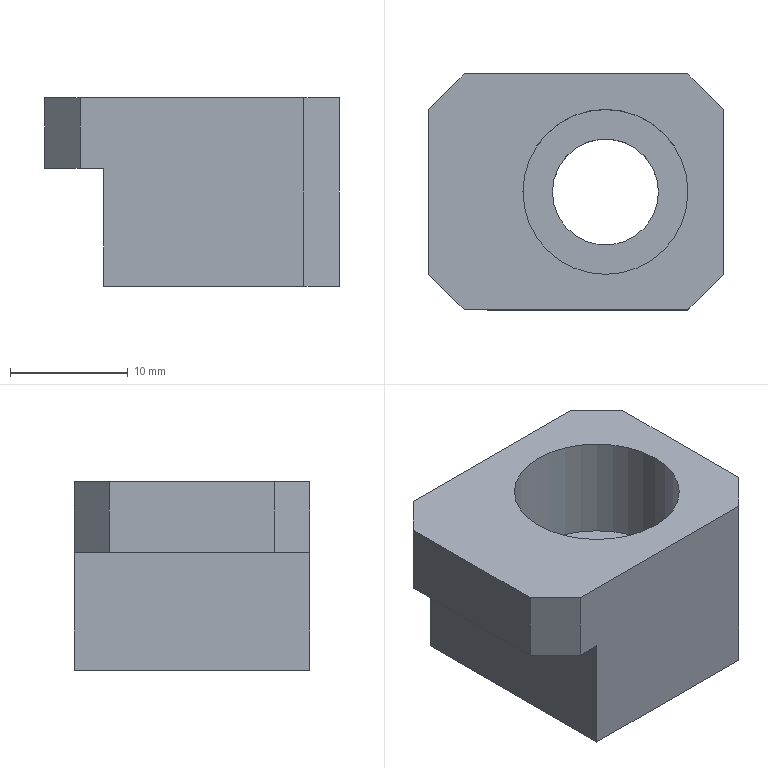Part | STEP file | gslz 2016.10.28-10_id1570_x_t | 1 solid | 15 faces | box 25 x 20 x 16 mm | volume 4971 mm3 | plane 13 | cylinder 2 | commonest cylinder face diameters 9 x1 14 x1
STEP:
#1=CARTESIAN_POINT('',(0.,0.,0.));
#2=DIRECTION('',(0.,0.,1.));
#3=DIRECTION('',(1.,0.,0.));
#4=AXIS2_PLACEMENT_3D('',#1,#2,#3);
#5=CARTESIAN_POINT('',(-846.5,210.,65.));
#6=VERTEX_POINT('',#5);
#7=CARTESIAN_POINT('',(-851.,210.,65.));
#8=DIRECTION('',(0.,0.,1.));
#9=DIRECTION('',(1.,0.,0.));
#10=AXIS2_PLACEMENT_3D('',#7,#8,#9);
#11=CIRCLE('',#10,4.5);
#12=CARTESIAN_POINT('',(-858.5,212.5,65.));
#13=DIRECTION('',(0.,0.,-1.));
#14=DIRECTION('',(1.,0.,0.));
#15=AXIS2_PLACEMENT_3D('',#12,#13,#14);
#16=PLANE('',#15);
#17=CARTESIAN_POINT('',(12.,2.5));
#18=CARTESIAN_POINT('',(12.,-5.294));
#19=CARTESIAN_POINT('',(5.25,-1.397));
#20=CARTESIAN_POINT('',(-1.5,2.5));
#21=CARTESIAN_POINT('',(5.25,6.397));
#22=CARTESIAN_POINT('',(12.,10.294));
#23=CARTESIAN_POINT('',(12.,2.5));
#24=(BOUNDED_CURVE()B_SPLINE_CURVE(2,(#17,#18,#19,#20,#21,#22,#23),.UNSPECIFIED.,.T.,.F.)B_SPLINE_CURVE_WITH_KNOTS((1,2,2,2,2,1),(-2.094,0.,2.094,4.189,6.283,8.378),.UNSPECIFIED.)CURVE()GEOMETRIC_REPRESENTATION_ITEM()RATIONAL_B_SPLINE_CURVE((1.,0.5,1.,0.5,1.,0.5,1.))REPRESENTATION_ITEM(''));
#25=(GEOMETRIC_REPRESENTATION_CONTEXT(2)PARAMETRIC_REPRESENTATION_CONTEXT()REPRESENTATION_CONTEXT('',''));
#26=DEFINITIONAL_REPRESENTATION('',(#24),#25);
#27=PCURVE('',#16,#26);
#28=CARTESIAN_POINT('',(-851.,210.,66.));
#29=DIRECTION('',(0.,0.,-1.));
#30=DIRECTION('',(0.,-1.,0.));
#31=AXIS2_PLACEMENT_3D('',#28,#29,#30);
#32=CYLINDRICAL_SURFACE('',#31,4.5);
#33=CARTESIAN_POINT('',(10.996,1.));
#34=DIRECTION('',(-1.,0.));
#35=VECTOR('',#34,1.);
#36=LINE('',#33,#35);
#37=(GEOMETRIC_REPRESENTATION_CONTEXT(2)PARAMETRIC_REPRESENTATION_CONTEXT()REPRESENTATION_CONTEXT('',''));
#38=DEFINITIONAL_REPRESENTATION('',(#36),#37);
#39=PCURVE('',#32,#38);
#40=SURFACE_CURVE('',#11,(#27,#39),.PCURVE_S1.);
#41=EDGE_CURVE('',#6,#6,#40,.T.);
#42=ORIENTED_EDGE('',*,*,#41,.T.);
#43=EDGE_LOOP('',(#42));
#44=FACE_BOUND('',#43,.T.);
#45=CARTESIAN_POINT('',(-841.,217.,65.));
#46=VERTEX_POINT('',#45);
#47=CARTESIAN_POINT('',(-841.,203.,65.));
#48=VERTEX_POINT('',#47);
#49=CARTESIAN_POINT('',(-841.,212.5,65.));
#50=DIRECTION('',(0.,-1.,0.));
#51=VECTOR('',#50,1.);
#52=LINE('',#49,#51);
#53=CARTESIAN_POINT('',(17.5,0.));
#54=DIRECTION('',(0.,1.));
#55=VECTOR('',#54,1.);
#56=LINE('',#53,#55);
#57=(GEOMETRIC_REPRESENTATION_CONTEXT(2)PARAMETRIC_REPRESENTATION_CONTEXT()REPRESENTATION_CONTEXT('',''));
#58=DEFINITIONAL_REPRESENTATION('',(#56),#57);
#59=PCURVE('',#16,#58);
#60=CARTESIAN_POINT('',(-841.,212.5,76.));
#61=DIRECTION('',(1.,0.,0.));
#62=DIRECTION('',(0.,0.,1.));
#63=AXIS2_PLACEMENT_3D('',#60,#61,#62);
#64=PLANE('',#63);
#65=CARTESIAN_POINT('',(-11.,0.));
#66=DIRECTION('',(0.,1.));
#67=VECTOR('',#66,1.);
#68=LINE('',#65,#67);
#69=(GEOMETRIC_REPRESENTATION_CONTEXT(2)PARAMETRIC_REPRESENTATION_CONTEXT()REPRESENTATION_CONTEXT('',''));
#70=DEFINITIONAL_REPRESENTATION('',(#68),#69);
#71=PCURVE('',#64,#70);
#72=SURFACE_CURVE('',#52,(#59,#71),.PCURVE_S1.);
#73=EDGE_CURVE('',#46,#48,#72,.T.);
#74=ORIENTED_EDGE('',*,*,#73,.T.);
#75=CARTESIAN_POINT('',(-844.,200.,65.));
#76=VERTEX_POINT('',#75);
#77=CARTESIAN_POINT('',(-845.,199.,65.));
#78=DIRECTION('',(0.7071,0.7071,0.));
#79=VECTOR('',#78,1.);
#80=LINE('',#77,#79);
#81=CARTESIAN_POINT('',(13.5,13.5));
#82=DIRECTION('',(0.7071,-0.7071));
#83=VECTOR('',#82,1.);
#84=LINE('',#81,#83);
#85=(GEOMETRIC_REPRESENTATION_CONTEXT(2)PARAMETRIC_REPRESENTATION_CONTEXT()REPRESENTATION_CONTEXT('',''));
#86=DEFINITIONAL_REPRESENTATION('',(#84),#85);
#87=PCURVE('',#16,#86);
#88=CARTESIAN_POINT('',(-841.,203.,76.));
#89=DIRECTION('',(-0.7071,0.7071,0.));
#90=DIRECTION('',(0.,0.,1.));
#91=AXIS2_PLACEMENT_3D('',#88,#89,#90);
#92=PLANE('',#91);
#93=CARTESIAN_POINT('',(-11.,-5.657));
#94=DIRECTION('',(0.,1.));
#95=VECTOR('',#94,1.);
#96=LINE('',#93,#95);
#97=(GEOMETRIC_REPRESENTATION_CONTEXT(2)PARAMETRIC_REPRESENTATION_CONTEXT()REPRESENTATION_CONTEXT('',''));
#98=DEFINITIONAL_REPRESENTATION('',(#96),#97);
#99=PCURVE('',#92,#98);
#100=SURFACE_CURVE('',#80,(#87,#99),.PCURVE_S1.);
#101=EDGE_CURVE('',#76,#48,#100,.T.);
#102=ORIENTED_EDGE('',*,*,#101,.F.);
#103=CARTESIAN_POINT('',(-861.,200.,65.));
#104=VERTEX_POINT('',#103);
#105=CARTESIAN_POINT('',(-858.5,200.,65.));
#106=DIRECTION('',(-1.,0.,0.));
#107=VECTOR('',#106,1.);
#108=LINE('',#105,#107);
#109=CARTESIAN_POINT('',(0.,12.5));
#110=DIRECTION('',(-1.,0.));
#111=VECTOR('',#110,1.);
#112=LINE('',#109,#111);
#113=(GEOMETRIC_REPRESENTATION_CONTEXT(2)PARAMETRIC_REPRESENTATION_CONTEXT()REPRESENTATION_CONTEXT('',''));
#114=DEFINITIONAL_REPRESENTATION('',(#112),#113);
#115=PCURVE('',#16,#114);
#116=CARTESIAN_POINT('',(-858.5,200.,76.));
#117=DIRECTION('',(0.,-1.,0.));
#118=DIRECTION('',(0.,0.,-1.));
#119=AXIS2_PLACEMENT_3D('',#116,#117,#118);
#120=PLANE('',#119);
#121=CARTESIAN_POINT('',(11.,0.));
#122=DIRECTION('',(0.,-1.));
#123=VECTOR('',#122,1.);
#124=LINE('',#121,#123);
#125=(GEOMETRIC_REPRESENTATION_CONTEXT(2)PARAMETRIC_REPRESENTATION_CONTEXT()REPRESENTATION_CONTEXT('',''));
#126=DEFINITIONAL_REPRESENTATION('',(#124),#125);
#127=PCURVE('',#120,#126);
#128=SURFACE_CURVE('',#108,(#115,#127),.PCURVE_S1.);
#129=EDGE_CURVE('',#76,#104,#128,.T.);
#130=ORIENTED_EDGE('',*,*,#129,.T.);
#131=CARTESIAN_POINT('',(-861.,220.,65.));
#132=VERTEX_POINT('',#131);
#133=CARTESIAN_POINT('',(-861.,212.5,65.));
#134=DIRECTION('',(0.,1.,0.));
#135=VECTOR('',#134,1.);
#136=LINE('',#133,#135);
#137=CARTESIAN_POINT('',(-2.5,0.));
#138=DIRECTION('',(0.,-1.));
#139=VECTOR('',#138,1.);
#140=LINE('',#137,#139);
#141=(GEOMETRIC_REPRESENTATION_CONTEXT(2)PARAMETRIC_REPRESENTATION_CONTEXT()REPRESENTATION_CONTEXT('',''));
#142=DEFINITIONAL_REPRESENTATION('',(#140),#141);
#143=PCURVE('',#16,#142);
#144=CARTESIAN_POINT('',(-861.,210.,76.));
#145=DIRECTION('',(1.,0.,0.));
#146=DIRECTION('',(0.,0.,1.));
#147=AXIS2_PLACEMENT_3D('',#144,#145,#146);
#148=PLANE('',#147);
#149=CARTESIAN_POINT('',(-11.,-2.5));
#150=DIRECTION('',(0.,-1.));
#151=VECTOR('',#150,1.);
#152=LINE('',#149,#151);
#153=(GEOMETRIC_REPRESENTATION_CONTEXT(2)PARAMETRIC_REPRESENTATION_CONTEXT()REPRESENTATION_CONTEXT('',''));
#154=DEFINITIONAL_REPRESENTATION('',(#152),#153);
#155=PCURVE('',#148,#154);
#156=SURFACE_CURVE('',#136,(#143,#155),.PCURVE_S1.);
#157=EDGE_CURVE('',#104,#132,#156,.T.);
#158=ORIENTED_EDGE('',*,*,#157,.T.);
#159=CARTESIAN_POINT('',(-844.,220.,65.));
#160=VERTEX_POINT('',#159);
#161=CARTESIAN_POINT('',(-858.5,220.,65.));
#162=DIRECTION('',(1.,0.,0.));
#163=VECTOR('',#162,1.);
#164=LINE('',#161,#163);
#165=CARTESIAN_POINT('',(0.,-7.5));
#166=DIRECTION('',(1.,0.));
#167=VECTOR('',#166,1.);
#168=LINE('',#165,#167);
#169=(GEOMETRIC_REPRESENTATION_CONTEXT(2)PARAMETRIC_REPRESENTATION_CONTEXT()REPRESENTATION_CONTEXT('',''));
#170=DEFINITIONAL_REPRESENTATION('',(#168),#169);
#171=PCURVE('',#16,#170);
#172=CARTESIAN_POINT('',(-858.5,220.,76.));
#173=DIRECTION('',(0.,1.,0.));
#174=DIRECTION('',(0.,0.,1.));
#175=AXIS2_PLACEMENT_3D('',#172,#173,#174);
#176=PLANE('',#175);
#177=CARTESIAN_POINT('',(-11.,0.));
#178=DIRECTION('',(0.,1.));
#179=VECTOR('',#178,1.);
#180=LINE('',#177,#179);
#181=(GEOMETRIC_REPRESENTATION_CONTEXT(2)PARAMETRIC_REPRESENTATION_CONTEXT()REPRESENTATION_CONTEXT('',''));
#182=DEFINITIONAL_REPRESENTATION('',(#180),#181);
#183=PCURVE('',#176,#182);
#184=SURFACE_CURVE('',#164,(#171,#183),.PCURVE_S1.);
#185=EDGE_CURVE('',#132,#160,#184,.T.);
#186=ORIENTED_EDGE('',*,*,#185,.T.);
#187=CARTESIAN_POINT('',(-847.5,223.5,65.));
#188=DIRECTION('',(-0.7071,0.7071,0.));
#189=VECTOR('',#188,1.);
#190=LINE('',#187,#189);
#191=CARTESIAN_POINT('',(11.,-11.));
#192=DIRECTION('',(-0.7071,-0.7071));
#193=VECTOR('',#192,1.);
#194=LINE('',#191,#193);
#195=(GEOMETRIC_REPRESENTATION_CONTEXT(2)PARAMETRIC_REPRESENTATION_CONTEXT()REPRESENTATION_CONTEXT('',''));
#196=DEFINITIONAL_REPRESENTATION('',(#194),#195);
#197=PCURVE('',#16,#196);
#198=CARTESIAN_POINT('',(-844.,220.,76.));
#199=DIRECTION('',(-0.7071,-0.7071,0.));
#200=DIRECTION('',(0.,0.,1.));
#201=AXIS2_PLACEMENT_3D('',#198,#199,#200);
#202=PLANE('',#201);
#203=CARTESIAN_POINT('',(-11.,4.95));
#204=DIRECTION('',(0.,1.));
#205=VECTOR('',#204,1.);
#206=LINE('',#203,#205);
#207=(GEOMETRIC_REPRESENTATION_CONTEXT(2)PARAMETRIC_REPRESENTATION_CONTEXT()REPRESENTATION_CONTEXT('',''));
#208=DEFINITIONAL_REPRESENTATION('',(#206),#207);
#209=PCURVE('',#202,#208);
#210=SURFACE_CURVE('',#190,(#197,#209),.PCURVE_S1.);
#211=EDGE_CURVE('',#46,#160,#210,.T.);
#212=ORIENTED_EDGE('',*,*,#211,.F.);
#213=EDGE_LOOP('',(#74,#102,#130,#158,#186,#212));
#214=FACE_BOUND('',#213,.T.);
#215=ADVANCED_FACE('',(#44,#214),#16,.T.);
#216=ORIENTED_EDGE('',*,*,#129,.F.);
#217=CARTESIAN_POINT('',(-844.,200.,81.));
#218=VERTEX_POINT('',#217);
#219=CARTESIAN_POINT('',(-844.,200.,76.));
#220=DIRECTION('',(0.,0.,-1.));
#221=VECTOR('',#220,1.);
#222=LINE('',#219,#221);
#223=CARTESIAN_POINT('',(0.,14.5));
#224=DIRECTION('',(1.,0.));
#225=VECTOR('',#224,1.);
#226=LINE('',#223,#225);
#227=(GEOMETRIC_REPRESENTATION_CONTEXT(2)PARAMETRIC_REPRESENTATION_CONTEXT()REPRESENTATION_CONTEXT('',''));
#228=DEFINITIONAL_REPRESENTATION('',(#226),#227);
#229=PCURVE('',#120,#228);
#230=CARTESIAN_POINT('',(0.,-4.243));
#231=DIRECTION('',(-1.,0.));
#232=VECTOR('',#231,1.);
#233=LINE('',#230,#232);
#234=(GEOMETRIC_REPRESENTATION_CONTEXT(2)PARAMETRIC_REPRESENTATION_CONTEXT()REPRESENTATION_CONTEXT('',''));
#235=DEFINITIONAL_REPRESENTATION('',(#233),#234);
#236=PCURVE('',#92,#235);
#237=SURFACE_CURVE('',#222,(#229,#236),.PCURVE_S1.);
#238=EDGE_CURVE('',#218,#76,#237,.T.);
#239=ORIENTED_EDGE('',*,*,#238,.F.);
#240=CARTESIAN_POINT('',(-863.,200.,81.));
#241=VERTEX_POINT('',#240);
#242=CARTESIAN_POINT('',(-858.5,200.,81.));
#243=DIRECTION('',(1.,0.,0.));
#244=VECTOR('',#243,1.);
#245=LINE('',#242,#244);
#246=CARTESIAN_POINT('',(-5.,0.));
#247=DIRECTION('',(0.,1.));
#248=VECTOR('',#247,1.);
#249=LINE('',#246,#248);
#250=(GEOMETRIC_REPRESENTATION_CONTEXT(2)PARAMETRIC_REPRESENTATION_CONTEXT()REPRESENTATION_CONTEXT('',''));
#251=DEFINITIONAL_REPRESENTATION('',(#249),#250);
#252=PCURVE('',#120,#251);
#253=CARTESIAN_POINT('',(-858.5,212.5,81.));
#254=DIRECTION('',(0.,0.,1.));
#255=DIRECTION('',(-1.,0.,0.));
#256=AXIS2_PLACEMENT_3D('',#253,#254,#255);
#257=PLANE('',#256);
#258=CARTESIAN_POINT('',(0.,12.5));
#259=DIRECTION('',(-1.,0.));
#260=VECTOR('',#259,1.);
#261=LINE('',#258,#260);
#262=(GEOMETRIC_REPRESENTATION_CONTEXT(2)PARAMETRIC_REPRESENTATION_CONTEXT()REPRESENTATION_CONTEXT('',''));
#263=DEFINITIONAL_REPRESENTATION('',(#261),#262);
#264=PCURVE('',#257,#263);
#265=SURFACE_CURVE('',#245,(#252,#264),.PCURVE_S1.);
#266=EDGE_CURVE('',#241,#218,#265,.T.);
#267=ORIENTED_EDGE('',*,*,#266,.F.);
#268=CARTESIAN_POINT('',(-863.,200.,75.));
#269=VERTEX_POINT('',#268);
#270=CARTESIAN_POINT('',(-863.,200.,76.));
#271=DIRECTION('',(0.,0.,1.));
#272=VECTOR('',#271,1.);
#273=LINE('',#270,#272);
#274=CARTESIAN_POINT('',(0.,-4.5));
#275=DIRECTION('',(-1.,0.));
#276=VECTOR('',#275,1.);
#277=LINE('',#274,#276);
#278=(GEOMETRIC_REPRESENTATION_CONTEXT(2)PARAMETRIC_REPRESENTATION_CONTEXT()REPRESENTATION_CONTEXT('',''));
#279=DEFINITIONAL_REPRESENTATION('',(#277),#278);
#280=PCURVE('',#120,#279);
#281=CARTESIAN_POINT('',(-863.,200.,76.));
#282=DIRECTION('',(0.7071,0.7071,0.));
#283=DIRECTION('',(0.,0.,1.));
#284=AXIS2_PLACEMENT_3D('',#281,#282,#283);
#285=PLANE('',#284);
#286=CARTESIAN_POINT('',(0.,0.));
#287=DIRECTION('',(1.,0.));
#288=VECTOR('',#287,1.);
#289=LINE('',#286,#288);
#290=(GEOMETRIC_REPRESENTATION_CONTEXT(2)PARAMETRIC_REPRESENTATION_CONTEXT()REPRESENTATION_CONTEXT('',''));
#291=DEFINITIONAL_REPRESENTATION('',(#289),#290);
#292=PCURVE('',#285,#291);
#293=SURFACE_CURVE('',#273,(#280,#292),.PCURVE_S1.);
#294=EDGE_CURVE('',#269,#241,#293,.T.);
#295=ORIENTED_EDGE('',*,*,#294,.F.);
#296=CARTESIAN_POINT('',(-861.,200.,75.));
#297=VERTEX_POINT('',#296);
#298=CARTESIAN_POINT('',(-858.5,200.,75.));
#299=DIRECTION('',(-1.,0.,0.));
#300=VECTOR('',#299,1.);
#301=LINE('',#298,#300);
#302=CARTESIAN_POINT('',(1.,0.));
#303=DIRECTION('',(0.,-1.));
#304=VECTOR('',#303,1.);
#305=LINE('',#302,#304);
#306=(GEOMETRIC_REPRESENTATION_CONTEXT(2)PARAMETRIC_REPRESENTATION_CONTEXT()REPRESENTATION_CONTEXT('',''));
#307=DEFINITIONAL_REPRESENTATION('',(#305),#306);
#308=PCURVE('',#120,#307);
#309=CARTESIAN_POINT('',(-883.5,210.,75.));
#310=DIRECTION('',(0.,0.,1.));
#311=DIRECTION('',(1.,0.,0.));
#312=AXIS2_PLACEMENT_3D('',#309,#310,#311);
#313=PLANE('',#312);
#314=CARTESIAN_POINT('',(25.,-10.));
#315=DIRECTION('',(-1.,0.));
#316=VECTOR('',#315,1.);
#317=LINE('',#314,#316);
#318=(GEOMETRIC_REPRESENTATION_CONTEXT(2)PARAMETRIC_REPRESENTATION_CONTEXT()REPRESENTATION_CONTEXT('',''));
#319=DEFINITIONAL_REPRESENTATION('',(#317),#318);
#320=PCURVE('',#313,#319);
#321=SURFACE_CURVE('',#301,(#308,#320),.PCURVE_S1.);
#322=EDGE_CURVE('',#297,#269,#321,.T.);
#323=ORIENTED_EDGE('',*,*,#322,.F.);
#324=CARTESIAN_POINT('',(-861.,200.,76.));
#325=DIRECTION('',(0.,0.,1.));
#326=VECTOR('',#325,1.);
#327=LINE('',#324,#326);
#328=CARTESIAN_POINT('',(0.,-2.5));
#329=DIRECTION('',(-1.,0.));
#330=VECTOR('',#329,1.);
#331=LINE('',#328,#330);
#332=(GEOMETRIC_REPRESENTATION_CONTEXT(2)PARAMETRIC_REPRESENTATION_CONTEXT()REPRESENTATION_CONTEXT('',''));
#333=DEFINITIONAL_REPRESENTATION('',(#331),#332);
#334=PCURVE('',#120,#333);
#335=CARTESIAN_POINT('',(0.,10.));
#336=DIRECTION('',(1.,0.));
#337=VECTOR('',#336,1.);
#338=LINE('',#335,#337);
#339=(GEOMETRIC_REPRESENTATION_CONTEXT(2)PARAMETRIC_REPRESENTATION_CONTEXT()REPRESENTATION_CONTEXT('',''));
#340=DEFINITIONAL_REPRESENTATION('',(#338),#339);
#341=PCURVE('',#148,#340);
#342=SURFACE_CURVE('',#327,(#334,#341),.PCURVE_S1.);
#343=EDGE_CURVE('',#104,#297,#342,.T.);
#344=ORIENTED_EDGE('',*,*,#343,.F.);
#345=EDGE_LOOP('',(#216,#239,#267,#295,#323,#344));
#346=FACE_BOUND('',#345,.T.);
#347=ADVANCED_FACE('',(#346),#120,.T.);
#348=CARTESIAN_POINT('',(-841.,203.,81.));
#349=VERTEX_POINT('',#348);
#350=CARTESIAN_POINT('',(-841.,217.,81.));
#351=VERTEX_POINT('',#350);
#352=CARTESIAN_POINT('',(-841.,212.5,81.));
#353=DIRECTION('',(0.,1.,0.));
#354=VECTOR('',#353,1.);
#355=LINE('',#352,#354);
#356=CARTESIAN_POINT('',(5.,0.));
#357=DIRECTION('',(0.,-1.));
#358=VECTOR('',#357,1.);
#359=LINE('',#356,#358);
#360=(GEOMETRIC_REPRESENTATION_CONTEXT(2)PARAMETRIC_REPRESENTATION_CONTEXT()REPRESENTATION_CONTEXT('',''));
#361=DEFINITIONAL_REPRESENTATION('',(#359),#360);
#362=PCURVE('',#64,#361);
#363=CARTESIAN_POINT('',(-17.5,0.));
#364=DIRECTION('',(0.,-1.));
#365=VECTOR('',#364,1.);
#366=LINE('',#363,#365);
#367=(GEOMETRIC_REPRESENTATION_CONTEXT(2)PARAMETRIC_REPRESENTATION_CONTEXT()REPRESENTATION_CONTEXT('',''));
#368=DEFINITIONAL_REPRESENTATION('',(#366),#367);
#369=PCURVE('',#257,#368);
#370=SURFACE_CURVE('',#355,(#362,#369),.PCURVE_S1.);
#371=EDGE_CURVE('',#349,#351,#370,.T.);
#372=ORIENTED_EDGE('',*,*,#371,.F.);
#373=CARTESIAN_POINT('',(-841.,203.,76.));
#374=DIRECTION('',(0.,0.,1.));
#375=VECTOR('',#374,1.);
#376=LINE('',#373,#375);
#377=CARTESIAN_POINT('',(0.,9.5));
#378=DIRECTION('',(1.,0.));
#379=VECTOR('',#378,1.);
#380=LINE('',#377,#379);
#381=(GEOMETRIC_REPRESENTATION_CONTEXT(2)PARAMETRIC_REPRESENTATION_CONTEXT()REPRESENTATION_CONTEXT('',''));
#382=DEFINITIONAL_REPRESENTATION('',(#380),#381);
#383=PCURVE('',#64,#382);
#384=CARTESIAN_POINT('',(0.,0.));
#385=DIRECTION('',(1.,0.));
#386=VECTOR('',#385,1.);
#387=LINE('',#384,#386);
#388=(GEOMETRIC_REPRESENTATION_CONTEXT(2)PARAMETRIC_REPRESENTATION_CONTEXT()REPRESENTATION_CONTEXT('',''));
#389=DEFINITIONAL_REPRESENTATION('',(#387),#388);
#390=PCURVE('',#92,#389);
#391=SURFACE_CURVE('',#376,(#383,#390),.PCURVE_S1.);
#392=EDGE_CURVE('',#48,#349,#391,.T.);
#393=ORIENTED_EDGE('',*,*,#392,.F.);
#394=ORIENTED_EDGE('',*,*,#73,.F.);
#395=CARTESIAN_POINT('',(-841.,217.,76.));
#396=DIRECTION('',(0.,0.,-1.));
#397=VECTOR('',#396,1.);
#398=LINE('',#395,#397);
#399=CARTESIAN_POINT('',(0.,-4.5));
#400=DIRECTION('',(-1.,0.));
#401=VECTOR('',#400,1.);
#402=LINE('',#399,#401);
#403=(GEOMETRIC_REPRESENTATION_CONTEXT(2)PARAMETRIC_REPRESENTATION_CONTEXT()REPRESENTATION_CONTEXT('',''));
#404=DEFINITIONAL_REPRESENTATION('',(#402),#403);
#405=PCURVE('',#64,#404);
#406=CARTESIAN_POINT('',(0.,-4.243));
#407=DIRECTION('',(-1.,0.));
#408=VECTOR('',#407,1.);
#409=LINE('',#406,#408);
#410=(GEOMETRIC_REPRESENTATION_CONTEXT(2)PARAMETRIC_REPRESENTATION_CONTEXT()REPRESENTATION_CONTEXT('',''));
#411=DEFINITIONAL_REPRESENTATION('',(#409),#410);
#412=PCURVE('',#202,#411);
#413=SURFACE_CURVE('',#398,(#405,#412),.PCURVE_S1.);
#414=EDGE_CURVE('',#351,#46,#413,.T.);
#415=ORIENTED_EDGE('',*,*,#414,.F.);
#416=EDGE_LOOP('',(#372,#393,#394,#415));
#417=FACE_BOUND('',#416,.T.);
#418=ADVANCED_FACE('',(#417),#64,.T.);
#419=CARTESIAN_POINT('',(-863.,220.,75.));
#420=VERTEX_POINT('',#419);
#421=CARTESIAN_POINT('',(-861.,220.,75.));
#422=VERTEX_POINT('',#421);
#423=CARTESIAN_POINT('',(-858.5,220.,75.));
#424=DIRECTION('',(1.,0.,0.));
#425=VECTOR('',#424,1.);
#426=LINE('',#423,#425);
#427=CARTESIAN_POINT('',(-1.,0.));
#428=DIRECTION('',(0.,1.));
#429=VECTOR('',#428,1.);
#430=LINE('',#427,#429);
#431=(GEOMETRIC_REPRESENTATION_CONTEXT(2)PARAMETRIC_REPRESENTATION_CONTEXT()REPRESENTATION_CONTEXT('',''));
#432=DEFINITIONAL_REPRESENTATION('',(#430),#431);
#433=PCURVE('',#176,#432);
#434=CARTESIAN_POINT('',(25.,10.));
#435=DIRECTION('',(1.,0.));
#436=VECTOR('',#435,1.);
#437=LINE('',#434,#436);
#438=(GEOMETRIC_REPRESENTATION_CONTEXT(2)PARAMETRIC_REPRESENTATION_CONTEXT()REPRESENTATION_CONTEXT('',''));
#439=DEFINITIONAL_REPRESENTATION('',(#437),#438);
#440=PCURVE('',#313,#439);
#441=SURFACE_CURVE('',#426,(#433,#440),.PCURVE_S1.);
#442=EDGE_CURVE('',#420,#422,#441,.T.);
#443=ORIENTED_EDGE('',*,*,#442,.F.);
#444=CARTESIAN_POINT('',(-863.,220.,81.));
#445=VERTEX_POINT('',#444);
#446=CARTESIAN_POINT('',(-863.,220.,76.));
#447=DIRECTION('',(0.,0.,-1.));
#448=VECTOR('',#447,1.);
#449=LINE('',#446,#448);
#450=CARTESIAN_POINT('',(0.,-4.5));
#451=DIRECTION('',(-1.,0.));
#452=VECTOR('',#451,1.);
#453=LINE('',#450,#452);
#454=(GEOMETRIC_REPRESENTATION_CONTEXT(2)PARAMETRIC_REPRESENTATION_CONTEXT()REPRESENTATION_CONTEXT('',''));
#455=DEFINITIONAL_REPRESENTATION('',(#453),#454);
#456=PCURVE('',#176,#455);
#457=CARTESIAN_POINT('',(-866.,217.,76.));
#458=DIRECTION('',(0.7071,-0.7071,0.));
#459=DIRECTION('',(0.,0.,1.));
#460=AXIS2_PLACEMENT_3D('',#457,#458,#459);
#461=PLANE('',#460);
#462=CARTESIAN_POINT('',(0.,-4.243));
#463=DIRECTION('',(-1.,0.));
#464=VECTOR('',#463,1.);
#465=LINE('',#462,#464);
#466=(GEOMETRIC_REPRESENTATION_CONTEXT(2)PARAMETRIC_REPRESENTATION_CONTEXT()REPRESENTATION_CONTEXT('',''));
#467=DEFINITIONAL_REPRESENTATION('',(#465),#466);
#468=PCURVE('',#461,#467);
#469=SURFACE_CURVE('',#449,(#456,#468),.PCURVE_S1.);
#470=EDGE_CURVE('',#445,#420,#469,.T.);
#471=ORIENTED_EDGE('',*,*,#470,.F.);
#472=CARTESIAN_POINT('',(-844.,220.,81.));
#473=VERTEX_POINT('',#472);
#474=CARTESIAN_POINT('',(-858.5,220.,81.));
#475=DIRECTION('',(-1.,0.,0.));
#476=VECTOR('',#475,1.);
#477=LINE('',#474,#476);
#478=CARTESIAN_POINT('',(5.,0.));
#479=DIRECTION('',(0.,-1.));
#480=VECTOR('',#479,1.);
#481=LINE('',#478,#480);
#482=(GEOMETRIC_REPRESENTATION_CONTEXT(2)PARAMETRIC_REPRESENTATION_CONTEXT()REPRESENTATION_CONTEXT('',''));
#483=DEFINITIONAL_REPRESENTATION('',(#481),#482);
#484=PCURVE('',#176,#483);
#485=CARTESIAN_POINT('',(0.,-7.5));
#486=DIRECTION('',(1.,0.));
#487=VECTOR('',#486,1.);
#488=LINE('',#485,#487);
#489=(GEOMETRIC_REPRESENTATION_CONTEXT(2)PARAMETRIC_REPRESENTATION_CONTEXT()REPRESENTATION_CONTEXT('',''));
#490=DEFINITIONAL_REPRESENTATION('',(#488),#489);
#491=PCURVE('',#257,#490);
#492=SURFACE_CURVE('',#477,(#484,#491),.PCURVE_S1.);
#493=EDGE_CURVE('',#473,#445,#492,.T.);
#494=ORIENTED_EDGE('',*,*,#493,.F.);
#495=CARTESIAN_POINT('',(-844.,220.,76.));
#496=DIRECTION('',(0.,0.,1.));
#497=VECTOR('',#496,1.);
#498=LINE('',#495,#497);
#499=CARTESIAN_POINT('',(0.,14.5));
#500=DIRECTION('',(1.,0.));
#501=VECTOR('',#500,1.);
#502=LINE('',#499,#501);
#503=(GEOMETRIC_REPRESENTATION_CONTEXT(2)PARAMETRIC_REPRESENTATION_CONTEXT()REPRESENTATION_CONTEXT('',''));
#504=DEFINITIONAL_REPRESENTATION('',(#502),#503);
#505=PCURVE('',#176,#504);
#506=CARTESIAN_POINT('',(0.,0.));
#507=DIRECTION('',(1.,0.));
#508=VECTOR('',#507,1.);
#509=LINE('',#506,#508);
#510=(GEOMETRIC_REPRESENTATION_CONTEXT(2)PARAMETRIC_REPRESENTATION_CONTEXT()REPRESENTATION_CONTEXT('',''));
#511=DEFINITIONAL_REPRESENTATION('',(#509),#510);
#512=PCURVE('',#202,#511);
#513=SURFACE_CURVE('',#498,(#505,#512),.PCURVE_S1.);
#514=EDGE_CURVE('',#160,#473,#513,.T.);
#515=ORIENTED_EDGE('',*,*,#514,.F.);
#516=ORIENTED_EDGE('',*,*,#185,.F.);
#517=CARTESIAN_POINT('',(-861.,220.,76.));
#518=DIRECTION('',(0.,0.,-1.));
#519=VECTOR('',#518,1.);
#520=LINE('',#517,#519);
#521=CARTESIAN_POINT('',(0.,-2.5));
#522=DIRECTION('',(-1.,0.));
#523=VECTOR('',#522,1.);
#524=LINE('',#521,#523);
#525=(GEOMETRIC_REPRESENTATION_CONTEXT(2)PARAMETRIC_REPRESENTATION_CONTEXT()REPRESENTATION_CONTEXT('',''));
#526=DEFINITIONAL_REPRESENTATION('',(#524),#525);
#527=PCURVE('',#176,#526);
#528=CARTESIAN_POINT('',(0.,-10.));
#529=DIRECTION('',(-1.,0.));
#530=VECTOR('',#529,1.);
#531=LINE('',#528,#530);
#532=(GEOMETRIC_REPRESENTATION_CONTEXT(2)PARAMETRIC_REPRESENTATION_CONTEXT()REPRESENTATION_CONTEXT('',''));
#533=DEFINITIONAL_REPRESENTATION('',(#531),#532);
#534=PCURVE('',#148,#533);
#535=SURFACE_CURVE('',#520,(#527,#534),.PCURVE_S1.);
#536=EDGE_CURVE('',#422,#132,#535,.T.);
#537=ORIENTED_EDGE('',*,*,#536,.F.);
#538=EDGE_LOOP('',(#443,#471,#494,#515,#516,#537));
#539=FACE_BOUND('',#538,.T.);
#540=ADVANCED_FACE('',(#539),#176,.T.);
#541=CARTESIAN_POINT('',(-858.,210.,81.));
#542=VERTEX_POINT('',#541);
#543=CARTESIAN_POINT('',(-844.,210.,81.));
#544=VERTEX_POINT('',#543);
#545=CARTESIAN_POINT('',(-851.,210.,81.));
#546=DIRECTION('',(0.,0.,-1.));
#547=DIRECTION('',(-1.,0.,0.));
#548=AXIS2_PLACEMENT_3D('',#545,#546,#547);
#549=CIRCLE('',#548,7.);
#550=CARTESIAN_POINT('',(-0.5,2.5));
#551=CARTESIAN_POINT('',(-0.5,-9.624));
#552=CARTESIAN_POINT('',(-11.,-3.562));
#553=CARTESIAN_POINT('',(-21.5,2.5));
#554=CARTESIAN_POINT('',(-11.,8.562));
#555=CARTESIAN_POINT('',(-0.5,14.624));
#556=CARTESIAN_POINT('',(-0.5,2.5));
#557=(BOUNDED_CURVE()B_SPLINE_CURVE(2,(#550,#551,#552,#553,#554,#555,#556),.UNSPECIFIED.,.T.,.F.)B_SPLINE_CURVE_WITH_KNOTS((1,2,2,2,2,1),(-2.094,0.,2.094,4.189,6.283,8.378),.UNSPECIFIED.)CURVE()GEOMETRIC_REPRESENTATION_ITEM()RATIONAL_B_SPLINE_CURVE((1.,0.5,1.,0.5,1.,0.5,1.))REPRESENTATION_ITEM(''));
#558=(GEOMETRIC_REPRESENTATION_CONTEXT(2)PARAMETRIC_REPRESENTATION_CONTEXT()REPRESENTATION_CONTEXT('',''));
#559=DEFINITIONAL_REPRESENTATION('',(#557),#558);
#560=PCURVE('',#257,#559);
#561=CARTESIAN_POINT('',(-851.,210.,86.));
#562=DIRECTION('',(0.,0.,-1.));
#563=DIRECTION('',(1.,0.,0.));
#564=AXIS2_PLACEMENT_3D('',#561,#562,#563);
#565=CYLINDRICAL_SURFACE('',#564,7.);
#566=CARTESIAN_POINT('',(3.142,5.));
#567=DIRECTION('',(1.,0.));
#568=VECTOR('',#567,1.);
#569=LINE('',#566,#568);
#570=(GEOMETRIC_REPRESENTATION_CONTEXT(2)PARAMETRIC_REPRESENTATION_CONTEXT()REPRESENTATION_CONTEXT('',''));
#571=DEFINITIONAL_REPRESENTATION('',(#569),#570);
#572=PCURVE('',#565,#571);
#573=SURFACE_CURVE('',#549,(#560,#572),.PCURVE_S1.);
#574=EDGE_CURVE('',#542,#544,#573,.T.);
#575=ORIENTED_EDGE('',*,*,#574,.T.);
#576=CARTESIAN_POINT('',(-851.,210.,81.));
#577=DIRECTION('',(0.,0.,-1.));
#578=DIRECTION('',(-1.,0.,0.));
#579=AXIS2_PLACEMENT_3D('',#576,#577,#578);
#580=CIRCLE('',#579,7.);
#581=CARTESIAN_POINT('',(-0.5,2.5));
#582=CARTESIAN_POINT('',(-0.5,-9.624));
#583=CARTESIAN_POINT('',(-11.,-3.562));
#584=CARTESIAN_POINT('',(-21.5,2.5));
#585=CARTESIAN_POINT('',(-11.,8.562));
#586=CARTESIAN_POINT('',(-0.5,14.624));
#587=CARTESIAN_POINT('',(-0.5,2.5));
#588=(BOUNDED_CURVE()B_SPLINE_CURVE(2,(#581,#582,#583,#584,#585,#586,#587),.UNSPECIFIED.,.T.,.F.)B_SPLINE_CURVE_WITH_KNOTS((1,2,2,2,2,1),(-2.094,0.,2.094,4.189,6.283,8.378),.UNSPECIFIED.)CURVE()GEOMETRIC_REPRESENTATION_ITEM()RATIONAL_B_SPLINE_CURVE((1.,0.5,1.,0.5,1.,0.5,1.))REPRESENTATION_ITEM(''));
#589=(GEOMETRIC_REPRESENTATION_CONTEXT(2)PARAMETRIC_REPRESENTATION_CONTEXT()REPRESENTATION_CONTEXT('',''));
#590=DEFINITIONAL_REPRESENTATION('',(#588),#589);
#591=PCURVE('',#257,#590);
#592=CARTESIAN_POINT('',(-3.142,5.));
#593=DIRECTION('',(1.,0.));
#594=VECTOR('',#593,1.);
#595=LINE('',#592,#594);
#596=(GEOMETRIC_REPRESENTATION_CONTEXT(2)PARAMETRIC_REPRESENTATION_CONTEXT()REPRESENTATION_CONTEXT('',''));
#597=DEFINITIONAL_REPRESENTATION('',(#595),#596);
#598=PCURVE('',#565,#597);
#599=SURFACE_CURVE('',#580,(#591,#598),.PCURVE_S1.);
#600=EDGE_CURVE('',#544,#542,#599,.T.);
#601=ORIENTED_EDGE('',*,*,#600,.T.);
#602=EDGE_LOOP('',(#575,#601));
#603=FACE_BOUND('',#602,.T.);
#604=ORIENTED_EDGE('',*,*,#266,.T.);
#605=CARTESIAN_POINT('',(-845.,199.,81.));
#606=DIRECTION('',(-0.7071,-0.7071,0.));
#607=VECTOR('',#606,1.);
#608=LINE('',#605,#607);
#609=CARTESIAN_POINT('',(-13.5,13.5));
#610=DIRECTION('',(0.7071,0.7071));
#611=VECTOR('',#610,1.);
#612=LINE('',#609,#611);
#613=(GEOMETRIC_REPRESENTATION_CONTEXT(2)PARAMETRIC_REPRESENTATION_CONTEXT()REPRESENTATION_CONTEXT('',''));
#614=DEFINITIONAL_REPRESENTATION('',(#612),#613);
#615=PCURVE('',#257,#614);
#616=CARTESIAN_POINT('',(5.,-5.657));
#617=DIRECTION('',(0.,-1.));
#618=VECTOR('',#617,1.);
#619=LINE('',#616,#618);
#620=(GEOMETRIC_REPRESENTATION_CONTEXT(2)PARAMETRIC_REPRESENTATION_CONTEXT()REPRESENTATION_CONTEXT('',''));
#621=DEFINITIONAL_REPRESENTATION('',(#619),#620);
#622=PCURVE('',#92,#621);
#623=SURFACE_CURVE('',#608,(#615,#622),.PCURVE_S1.);
#624=EDGE_CURVE('',#349,#218,#623,.T.);
#625=ORIENTED_EDGE('',*,*,#624,.F.);
#626=ORIENTED_EDGE('',*,*,#371,.T.);
#627=CARTESIAN_POINT('',(-847.5,223.5,81.));
#628=DIRECTION('',(0.7071,-0.7071,0.));
#629=VECTOR('',#628,1.);
#630=LINE('',#627,#629);
#631=CARTESIAN_POINT('',(-11.,-11.));
#632=DIRECTION('',(-0.7071,0.7071));
#633=VECTOR('',#632,1.);
#634=LINE('',#631,#633);
#635=(GEOMETRIC_REPRESENTATION_CONTEXT(2)PARAMETRIC_REPRESENTATION_CONTEXT()REPRESENTATION_CONTEXT('',''));
#636=DEFINITIONAL_REPRESENTATION('',(#634),#635);
#637=PCURVE('',#257,#636);
#638=CARTESIAN_POINT('',(5.,4.95));
#639=DIRECTION('',(0.,-1.));
#640=VECTOR('',#639,1.);
#641=LINE('',#638,#640);
#642=(GEOMETRIC_REPRESENTATION_CONTEXT(2)PARAMETRIC_REPRESENTATION_CONTEXT()REPRESENTATION_CONTEXT('',''));
#643=DEFINITIONAL_REPRESENTATION('',(#641),#642);
#644=PCURVE('',#202,#643);
#645=SURFACE_CURVE('',#630,(#637,#644),.PCURVE_S1.);
#646=EDGE_CURVE('',#473,#351,#645,.T.);
#647=ORIENTED_EDGE('',*,*,#646,.F.);
#648=ORIENTED_EDGE('',*,*,#493,.T.);
#649=CARTESIAN_POINT('',(-866.,217.,81.));
#650=VERTEX_POINT('',#649);
#651=CARTESIAN_POINT('',(-864.5,218.5,81.));
#652=DIRECTION('',(0.7071,0.7071,0.));
#653=VECTOR('',#652,1.);
#654=LINE('',#651,#653);
#655=CARTESIAN_POINT('',(6.,-6.));
#656=DIRECTION('',(-0.7071,-0.7071));
#657=VECTOR('',#656,1.);
#658=LINE('',#655,#657);
#659=(GEOMETRIC_REPRESENTATION_CONTEXT(2)PARAMETRIC_REPRESENTATION_CONTEXT()REPRESENTATION_CONTEXT('',''));
#660=DEFINITIONAL_REPRESENTATION('',(#658),#659);
#661=PCURVE('',#257,#660);
#662=CARTESIAN_POINT('',(5.,-2.121));
#663=DIRECTION('',(0.,-1.));
#664=VECTOR('',#663,1.);
#665=LINE('',#662,#664);
#666=(GEOMETRIC_REPRESENTATION_CONTEXT(2)PARAMETRIC_REPRESENTATION_CONTEXT()REPRESENTATION_CONTEXT('',''));
#667=DEFINITIONAL_REPRESENTATION('',(#665),#666);
#668=PCURVE('',#461,#667);
#669=SURFACE_CURVE('',#654,(#661,#668),.PCURVE_S1.);
#670=EDGE_CURVE('',#650,#445,#669,.T.);
#671=ORIENTED_EDGE('',*,*,#670,.F.);
#672=CARTESIAN_POINT('',(-866.,203.,81.));
#673=VERTEX_POINT('',#672);
#674=CARTESIAN_POINT('',(-866.,212.5,81.));
#675=DIRECTION('',(0.,-1.,0.));
#676=VECTOR('',#675,1.);
#677=LINE('',#674,#676);
#678=CARTESIAN_POINT('',(7.5,0.));
#679=DIRECTION('',(0.,1.));
#680=VECTOR('',#679,1.);
#681=LINE('',#678,#680);
#682=(GEOMETRIC_REPRESENTATION_CONTEXT(2)PARAMETRIC_REPRESENTATION_CONTEXT()REPRESENTATION_CONTEXT('',''));
#683=DEFINITIONAL_REPRESENTATION('',(#681),#682);
#684=PCURVE('',#257,#683);
#685=CARTESIAN_POINT('',(-866.,212.5,76.));
#686=DIRECTION('',(-1.,0.,0.));
#687=DIRECTION('',(0.,0.,-1.));
#688=AXIS2_PLACEMENT_3D('',#685,#686,#687);
#689=PLANE('',#688);
#690=CARTESIAN_POINT('',(-5.,0.));
#691=DIRECTION('',(0.,1.));
#692=VECTOR('',#691,1.);
#693=LINE('',#690,#692);
#694=(GEOMETRIC_REPRESENTATION_CONTEXT(2)PARAMETRIC_REPRESENTATION_CONTEXT()REPRESENTATION_CONTEXT('',''));
#695=DEFINITIONAL_REPRESENTATION('',(#693),#694);
#696=PCURVE('',#689,#695);
#697=SURFACE_CURVE('',#677,(#684,#696),.PCURVE_S1.);
#698=EDGE_CURVE('',#650,#673,#697,.T.);
#699=ORIENTED_EDGE('',*,*,#698,.T.);
#700=CARTESIAN_POINT('',(-867.,204.,81.));
#701=DIRECTION('',(-0.7071,0.7071,0.));
#702=VECTOR('',#701,1.);
#703=LINE('',#700,#702);
#704=CARTESIAN_POINT('',(8.5,8.5));
#705=DIRECTION('',(0.7071,-0.7071));
#706=VECTOR('',#705,1.);
#707=LINE('',#704,#706);
#708=(GEOMETRIC_REPRESENTATION_CONTEXT(2)PARAMETRIC_REPRESENTATION_CONTEXT()REPRESENTATION_CONTEXT('',''));
#709=DEFINITIONAL_REPRESENTATION('',(#707),#708);
#710=PCURVE('',#257,#709);
#711=CARTESIAN_POINT('',(5.,-5.657));
#712=DIRECTION('',(0.,-1.));
#713=VECTOR('',#712,1.);
#714=LINE('',#711,#713);
#715=(GEOMETRIC_REPRESENTATION_CONTEXT(2)PARAMETRIC_REPRESENTATION_CONTEXT()REPRESENTATION_CONTEXT('',''));
#716=DEFINITIONAL_REPRESENTATION('',(#714),#715);
#717=PCURVE('',#285,#716);
#718=SURFACE_CURVE('',#703,(#710,#717),.PCURVE_S1.);
#719=EDGE_CURVE('',#241,#673,#718,.T.);
#720=ORIENTED_EDGE('',*,*,#719,.F.);
#721=EDGE_LOOP('',(#604,#625,#626,#647,#648,#671,#699,#720));
#722=FACE_BOUND('',#721,.T.);
#723=ADVANCED_FACE('',(#603,#722),#257,.T.);
#724=ORIENTED_EDGE('',*,*,#343,.T.);
#725=CARTESIAN_POINT('',(-861.,210.,75.));
#726=DIRECTION('',(0.,-1.,0.));
#727=VECTOR('',#726,1.);
#728=LINE('',#725,#727);
#729=CARTESIAN_POINT('',(-1.,0.));
#730=DIRECTION('',(0.,1.));
#731=VECTOR('',#730,1.);
#732=LINE('',#729,#731);
#733=(GEOMETRIC_REPRESENTATION_CONTEXT(2)PARAMETRIC_REPRESENTATION_CONTEXT()REPRESENTATION_CONTEXT('',''));
#734=DEFINITIONAL_REPRESENTATION('',(#732),#733);
#735=PCURVE('',#148,#734);
#736=CARTESIAN_POINT('',(22.5,0.));
#737=DIRECTION('',(0.,-1.));
#738=VECTOR('',#737,1.);
#739=LINE('',#736,#738);
#740=(GEOMETRIC_REPRESENTATION_CONTEXT(2)PARAMETRIC_REPRESENTATION_CONTEXT()REPRESENTATION_CONTEXT('',''));
#741=DEFINITIONAL_REPRESENTATION('',(#739),#740);
#742=PCURVE('',#313,#741);
#743=SURFACE_CURVE('',#728,(#735,#742),.PCURVE_S1.);
#744=EDGE_CURVE('',#422,#297,#743,.T.);
#745=ORIENTED_EDGE('',*,*,#744,.F.);
#746=ORIENTED_EDGE('',*,*,#536,.T.);
#747=ORIENTED_EDGE('',*,*,#157,.F.);
#748=EDGE_LOOP('',(#724,#745,#746,#747));
#749=FACE_BOUND('',#748,.T.);
#750=ADVANCED_FACE('',(#749),#148,.F.);
#751=ORIENTED_EDGE('',*,*,#698,.F.);
#752=CARTESIAN_POINT('',(-866.,217.,75.));
#753=VERTEX_POINT('',#752);
#754=CARTESIAN_POINT('',(-866.,217.,76.));
#755=DIRECTION('',(0.,0.,1.));
#756=VECTOR('',#755,1.);
#757=LINE('',#754,#756);
#758=CARTESIAN_POINT('',(0.,-4.5));
#759=DIRECTION('',(-1.,0.));
#760=VECTOR('',#759,1.);
#761=LINE('',#758,#760);
#762=(GEOMETRIC_REPRESENTATION_CONTEXT(2)PARAMETRIC_REPRESENTATION_CONTEXT()REPRESENTATION_CONTEXT('',''));
#763=DEFINITIONAL_REPRESENTATION('',(#761),#762);
#764=PCURVE('',#689,#763);
#765=CARTESIAN_POINT('',(0.,0.));
#766=DIRECTION('',(1.,0.));
#767=VECTOR('',#766,1.);
#768=LINE('',#765,#767);
#769=(GEOMETRIC_REPRESENTATION_CONTEXT(2)PARAMETRIC_REPRESENTATION_CONTEXT()REPRESENTATION_CONTEXT('',''));
#770=DEFINITIONAL_REPRESENTATION('',(#768),#769);
#771=PCURVE('',#461,#770);
#772=SURFACE_CURVE('',#757,(#764,#771),.PCURVE_S1.);
#773=EDGE_CURVE('',#753,#650,#772,.T.);
#774=ORIENTED_EDGE('',*,*,#773,.F.);
#775=CARTESIAN_POINT('',(-866.,203.,75.));
#776=VERTEX_POINT('',#775);
#777=CARTESIAN_POINT('',(-866.,212.5,75.));
#778=DIRECTION('',(0.,1.,0.));
#779=VECTOR('',#778,1.);
#780=LINE('',#777,#779);
#781=CARTESIAN_POINT('',(1.,0.));
#782=DIRECTION('',(0.,-1.));
#783=VECTOR('',#782,1.);
#784=LINE('',#781,#783);
#785=(GEOMETRIC_REPRESENTATION_CONTEXT(2)PARAMETRIC_REPRESENTATION_CONTEXT()REPRESENTATION_CONTEXT('',''));
#786=DEFINITIONAL_REPRESENTATION('',(#784),#785);
#787=PCURVE('',#689,#786);
#788=CARTESIAN_POINT('',(17.5,2.5));
#789=DIRECTION('',(0.,1.));
#790=VECTOR('',#789,1.);
#791=LINE('',#788,#790);
#792=(GEOMETRIC_REPRESENTATION_CONTEXT(2)PARAMETRIC_REPRESENTATION_CONTEXT()REPRESENTATION_CONTEXT('',''));
#793=DEFINITIONAL_REPRESENTATION('',(#791),#792);
#794=PCURVE('',#313,#793);
#795=SURFACE_CURVE('',#780,(#787,#794),.PCURVE_S1.);
#796=EDGE_CURVE('',#776,#753,#795,.T.);
#797=ORIENTED_EDGE('',*,*,#796,.F.);
#798=CARTESIAN_POINT('',(-866.,203.,76.));
#799=DIRECTION('',(0.,0.,-1.));
#800=VECTOR('',#799,1.);
#801=LINE('',#798,#800);
#802=CARTESIAN_POINT('',(0.,9.5));
#803=DIRECTION('',(1.,0.));
#804=VECTOR('',#803,1.);
#805=LINE('',#802,#804);
#806=(GEOMETRIC_REPRESENTATION_CONTEXT(2)PARAMETRIC_REPRESENTATION_CONTEXT()REPRESENTATION_CONTEXT('',''));
#807=DEFINITIONAL_REPRESENTATION('',(#805),#806);
#808=PCURVE('',#689,#807);
#809=CARTESIAN_POINT('',(0.,-4.243));
#810=DIRECTION('',(-1.,0.));
#811=VECTOR('',#810,1.);
#812=LINE('',#809,#811);
#813=(GEOMETRIC_REPRESENTATION_CONTEXT(2)PARAMETRIC_REPRESENTATION_CONTEXT()REPRESENTATION_CONTEXT('',''));
#814=DEFINITIONAL_REPRESENTATION('',(#812),#813);
#815=PCURVE('',#285,#814);
#816=SURFACE_CURVE('',#801,(#808,#815),.PCURVE_S1.);
#817=EDGE_CURVE('',#673,#776,#816,.T.);
#818=ORIENTED_EDGE('',*,*,#817,.F.);
#819=EDGE_LOOP('',(#751,#774,#797,#818));
#820=FACE_BOUND('',#819,.T.);
#821=ADVANCED_FACE('',(#820),#689,.T.);
#822=ORIENTED_EDGE('',*,*,#796,.T.);
#823=CARTESIAN_POINT('',(-877.25,205.75,75.));
#824=DIRECTION('',(-0.7071,-0.7071,0.));
#825=VECTOR('',#824,1.);
#826=LINE('',#823,#825);
#827=CARTESIAN_POINT('',(6.25,-4.25));
#828=DIRECTION('',(-0.7071,-0.7071));
#829=VECTOR('',#828,1.);
#830=LINE('',#827,#829);
#831=(GEOMETRIC_REPRESENTATION_CONTEXT(2)PARAMETRIC_REPRESENTATION_CONTEXT()REPRESENTATION_CONTEXT('',''));
#832=DEFINITIONAL_REPRESENTATION('',(#830),#831);
#833=PCURVE('',#313,#832);
#834=CARTESIAN_POINT('',(-1.,15.91));
#835=DIRECTION('',(0.,1.));
#836=VECTOR('',#835,1.);
#837=LINE('',#834,#836);
#838=(GEOMETRIC_REPRESENTATION_CONTEXT(2)PARAMETRIC_REPRESENTATION_CONTEXT()REPRESENTATION_CONTEXT('',''));
#839=DEFINITIONAL_REPRESENTATION('',(#837),#838);
#840=PCURVE('',#461,#839);
#841=SURFACE_CURVE('',#826,(#833,#840),.PCURVE_S1.);
#842=EDGE_CURVE('',#420,#753,#841,.T.);
#843=ORIENTED_EDGE('',*,*,#842,.F.);
#844=ORIENTED_EDGE('',*,*,#442,.T.);
#845=ORIENTED_EDGE('',*,*,#744,.T.);
#846=ORIENTED_EDGE('',*,*,#322,.T.);
#847=CARTESIAN_POINT('',(-877.25,214.25,75.));
#848=DIRECTION('',(0.7071,-0.7071,0.));
#849=VECTOR('',#848,1.);
#850=LINE('',#847,#849);
#851=CARTESIAN_POINT('',(6.25,4.25));
#852=DIRECTION('',(0.7071,-0.7071));
#853=VECTOR('',#852,1.);
#854=LINE('',#851,#853);
#855=(GEOMETRIC_REPRESENTATION_CONTEXT(2)PARAMETRIC_REPRESENTATION_CONTEXT()REPRESENTATION_CONTEXT('',''));
#856=DEFINITIONAL_REPRESENTATION('',(#854),#855);
#857=PCURVE('',#313,#856);
#858=CARTESIAN_POINT('',(-1.,-20.153));
#859=DIRECTION('',(0.,1.));
#860=VECTOR('',#859,1.);
#861=LINE('',#858,#860);
#862=(GEOMETRIC_REPRESENTATION_CONTEXT(2)PARAMETRIC_REPRESENTATION_CONTEXT()REPRESENTATION_CONTEXT('',''));
#863=DEFINITIONAL_REPRESENTATION('',(#861),#862);
#864=PCURVE('',#285,#863);
#865=SURFACE_CURVE('',#850,(#857,#864),.PCURVE_S1.);
#866=EDGE_CURVE('',#776,#269,#865,.T.);
#867=ORIENTED_EDGE('',*,*,#866,.F.);
#868=EDGE_LOOP('',(#822,#843,#844,#845,#846,#867));
#869=FACE_BOUND('',#868,.T.);
#870=ADVANCED_FACE('',(#869),#313,.F.);
#871=ORIENTED_EDGE('',*,*,#574,.T.);
#872=CARTESIAN_POINT('',(-844.,210.,72.));
#873=VERTEX_POINT('',#872);
#874=CARTESIAN_POINT('',(-844.,210.,81.));
#875=CARTESIAN_POINT('',(-844.,210.,72.));
#876=B_SPLINE_CURVE_WITH_KNOTS('',1,(#874,#875),.UNSPECIFIED.,.F.,.F.,(2,2),(5.,14.),.PIECEWISE_BEZIER_KNOTS.);
#877=CARTESIAN_POINT('',(6.283,0.));
#878=DIRECTION('',(0.,1.));
#879=VECTOR('',#878,1.);
#880=LINE('',#877,#879);
#881=(GEOMETRIC_REPRESENTATION_CONTEXT(2)PARAMETRIC_REPRESENTATION_CONTEXT()REPRESENTATION_CONTEXT('',''));
#882=DEFINITIONAL_REPRESENTATION('',(#880),#881);
#883=PCURVE('',#565,#882);
#884=CARTESIAN_POINT('',(0.,0.));
#885=DIRECTION('',(0.,1.));
#886=VECTOR('',#885,1.);
#887=LINE('',#884,#886);
#888=(GEOMETRIC_REPRESENTATION_CONTEXT(2)PARAMETRIC_REPRESENTATION_CONTEXT()REPRESENTATION_CONTEXT('',''));
#889=DEFINITIONAL_REPRESENTATION('',(#887),#888);
#890=PCURVE('',#565,#889);
#891=SEAM_CURVE('',#876,(#883,#890),.PCURVE_S1.);
#892=EDGE_CURVE('',#544,#873,#891,.T.);
#893=ORIENTED_EDGE('',*,*,#892,.T.);
#894=CARTESIAN_POINT('',(-851.,210.,72.));
#895=DIRECTION('',(0.,0.,-1.));
#896=DIRECTION('',(1.,0.,0.));
#897=AXIS2_PLACEMENT_3D('',#894,#895,#896);
#898=CIRCLE('',#897,7.);
#899=CARTESIAN_POINT('',(0.,14.));
#900=DIRECTION('',(1.,0.));
#901=VECTOR('',#900,1.);
#902=LINE('',#899,#901);
#903=(GEOMETRIC_REPRESENTATION_CONTEXT(2)PARAMETRIC_REPRESENTATION_CONTEXT()REPRESENTATION_CONTEXT('',''));
#904=DEFINITIONAL_REPRESENTATION('',(#902),#903);
#905=PCURVE('',#565,#904);
#906=CARTESIAN_POINT('',(-851.,210.,72.));
#907=DIRECTION('',(0.,0.,-1.));
#908=DIRECTION('',(1.,0.,0.));
#909=AXIS2_PLACEMENT_3D('',#906,#907,#908);
#910=PLANE('',#909);
#911=CARTESIAN_POINT('',(0.,0.));
#912=DIRECTION('',(1.,0.));
#913=AXIS2_PLACEMENT_2D('',#911,#912);
#914=CIRCLE('',#913,7.);
#915=(GEOMETRIC_REPRESENTATION_CONTEXT(2)PARAMETRIC_REPRESENTATION_CONTEXT()REPRESENTATION_CONTEXT('',''));
#916=DEFINITIONAL_REPRESENTATION('',(#914),#915);
#917=PCURVE('',#910,#916);
#918=SURFACE_CURVE('',#898,(#905,#917),.PCURVE_S1.);
#919=EDGE_CURVE('',#873,#873,#918,.T.);
#920=ORIENTED_EDGE('',*,*,#919,.F.);
#921=ORIENTED_EDGE('',*,*,#892,.F.);
#922=ORIENTED_EDGE('',*,*,#600,.T.);
#923=EDGE_LOOP('',(#871,#893,#920,#921,#922));
#924=FACE_BOUND('',#923,.F.);
#925=ADVANCED_FACE('',(#924),#565,.F.);
#926=CARTESIAN_POINT('',(-846.5,210.,72.));
#927=VERTEX_POINT('',#926);
#928=CARTESIAN_POINT('',(-851.,210.,72.));
#929=DIRECTION('',(0.,0.,1.));
#930=DIRECTION('',(1.,0.,0.));
#931=AXIS2_PLACEMENT_3D('',#928,#929,#930);
#932=CIRCLE('',#931,4.5);
#933=CARTESIAN_POINT('',(4.5,0.));
#934=CARTESIAN_POINT('',(4.5,-7.794));
#935=CARTESIAN_POINT('',(-2.25,-3.897));
#936=CARTESIAN_POINT('',(-9.,0.));
#937=CARTESIAN_POINT('',(-2.25,3.897));
#938=CARTESIAN_POINT('',(4.5,7.794));
#939=CARTESIAN_POINT('',(4.5,0.));
#940=(BOUNDED_CURVE()B_SPLINE_CURVE(2,(#933,#934,#935,#936,#937,#938,#939),.UNSPECIFIED.,.T.,.F.)B_SPLINE_CURVE_WITH_KNOTS((1,2,2,2,2,1),(-2.094,0.,2.094,4.189,6.283,8.378),.UNSPECIFIED.)CURVE()GEOMETRIC_REPRESENTATION_ITEM()RATIONAL_B_SPLINE_CURVE((1.,0.5,1.,0.5,1.,0.5,1.))REPRESENTATION_ITEM(''));
#941=(GEOMETRIC_REPRESENTATION_CONTEXT(2)PARAMETRIC_REPRESENTATION_CONTEXT()REPRESENTATION_CONTEXT('',''));
#942=DEFINITIONAL_REPRESENTATION('',(#940),#941);
#943=PCURVE('',#910,#942);
#944=CARTESIAN_POINT('',(10.996,-6.));
#945=DIRECTION('',(-1.,0.));
#946=VECTOR('',#945,1.);
#947=LINE('',#944,#946);
#948=(GEOMETRIC_REPRESENTATION_CONTEXT(2)PARAMETRIC_REPRESENTATION_CONTEXT()REPRESENTATION_CONTEXT('',''));
#949=DEFINITIONAL_REPRESENTATION('',(#947),#948);
#950=PCURVE('',#32,#949);
#951=SURFACE_CURVE('',#932,(#943,#950),.PCURVE_S1.);
#952=EDGE_CURVE('',#927,#927,#951,.T.);
#953=ORIENTED_EDGE('',*,*,#952,.F.);
#954=EDGE_LOOP('',(#953));
#955=FACE_BOUND('',#954,.T.);
#956=ORIENTED_EDGE('',*,*,#919,.F.);
#957=EDGE_LOOP('',(#956));
#958=FACE_BOUND('',#957,.T.);
#959=ADVANCED_FACE('',(#955,#958),#910,.F.);
#960=ORIENTED_EDGE('',*,*,#41,.T.);
#961=CARTESIAN_POINT('',(-846.5,210.,72.));
#962=CARTESIAN_POINT('',(-846.5,210.,65.));
#963=B_SPLINE_CURVE_WITH_KNOTS('',1,(#961,#962),.UNSPECIFIED.,.F.,.F.,(2,2),(-6.,1.),.PIECEWISE_BEZIER_KNOTS.);
#964=CARTESIAN_POINT('',(4.712,0.));
#965=DIRECTION('',(0.,1.));
#966=VECTOR('',#965,1.);
#967=LINE('',#964,#966);
#968=(GEOMETRIC_REPRESENTATION_CONTEXT(2)PARAMETRIC_REPRESENTATION_CONTEXT()REPRESENTATION_CONTEXT('',''));
#969=DEFINITIONAL_REPRESENTATION('',(#967),#968);
#970=PCURVE('',#32,#969);
#971=CARTESIAN_POINT('',(10.996,0.));
#972=DIRECTION('',(0.,1.));
#973=VECTOR('',#972,1.);
#974=LINE('',#971,#973);
#975=(GEOMETRIC_REPRESENTATION_CONTEXT(2)PARAMETRIC_REPRESENTATION_CONTEXT()REPRESENTATION_CONTEXT('',''));
#976=DEFINITIONAL_REPRESENTATION('',(#974),#975);
#977=PCURVE('',#32,#976);
#978=SEAM_CURVE('',#963,(#970,#977),.PCURVE_S1.);
#979=EDGE_CURVE('',#927,#6,#978,.T.);
#980=ORIENTED_EDGE('',*,*,#979,.F.);
#981=ORIENTED_EDGE('',*,*,#952,.F.);
#982=ORIENTED_EDGE('',*,*,#979,.T.);
#983=EDGE_LOOP('',(#960,#980,#981,#982));
#984=FACE_BOUND('',#983,.F.);
#985=ADVANCED_FACE('',(#984),#32,.F.);
#986=ORIENTED_EDGE('',*,*,#624,.T.);
#987=ORIENTED_EDGE('',*,*,#238,.T.);
#988=ORIENTED_EDGE('',*,*,#101,.T.);
#989=ORIENTED_EDGE('',*,*,#392,.T.);
#990=EDGE_LOOP('',(#986,#987,#988,#989));
#991=FACE_BOUND('',#990,.T.);
#992=ADVANCED_FACE('',(#991),#92,.F.);
#993=ORIENTED_EDGE('',*,*,#670,.T.);
#994=ORIENTED_EDGE('',*,*,#470,.T.);
#995=ORIENTED_EDGE('',*,*,#842,.T.);
#996=ORIENTED_EDGE('',*,*,#773,.T.);
#997=EDGE_LOOP('',(#993,#994,#995,#996));
#998=FACE_BOUND('',#997,.T.);
#999=ADVANCED_FACE('',(#998),#461,.F.);
#1000=ORIENTED_EDGE('',*,*,#646,.T.);
#1001=ORIENTED_EDGE('',*,*,#414,.T.);
#1002=ORIENTED_EDGE('',*,*,#211,.T.);
#1003=ORIENTED_EDGE('',*,*,#514,.T.);
#1004=EDGE_LOOP('',(#1000,#1001,#1002,#1003));
#1005=FACE_BOUND('',#1004,.T.);
#1006=ADVANCED_FACE('',(#1005),#202,.F.);
#1007=ORIENTED_EDGE('',*,*,#719,.T.);
#1008=ORIENTED_EDGE('',*,*,#817,.T.);
#1009=ORIENTED_EDGE('',*,*,#866,.T.);
#1010=ORIENTED_EDGE('',*,*,#294,.T.);
#1011=EDGE_LOOP('',(#1007,#1008,#1009,#1010));
#1012=FACE_BOUND('',#1011,.T.);
#1013=ADVANCED_FACE('',(#1012),#285,.F.);
#1014=CLOSED_SHELL('',(#215,#347,#418,#540,#723,#750,#821,#870,#925,#959,#985,#992,#999,#1006,#1013));
#1015=MANIFOLD_SOLID_BREP('',#1014);
#1016=(LENGTH_UNIT()NAMED_UNIT(*)SI_UNIT(.MILLI.,.METRE.));
#1017=UNCERTAINTY_MEASURE_WITH_UNIT(LENGTH_MEASURE(0.000001),#1016,'','');
#1018=(NAMED_UNIT(*)PLANE_ANGLE_UNIT()SI_UNIT($,.RADIAN.));
#1019=(NAMED_UNIT(*)SI_UNIT($,.STERADIAN.)SOLID_ANGLE_UNIT());
#1020=(GEOMETRIC_REPRESENTATION_CONTEXT(3)GLOBAL_UNCERTAINTY_ASSIGNED_CONTEXT((#1017))GLOBAL_UNIT_ASSIGNED_CONTEXT((#1016,#1018,#1019))REPRESENTATION_CONTEXT('',''));
#1021=ADVANCED_BREP_SHAPE_REPRESENTATION('',(#4,#1015),#1020);